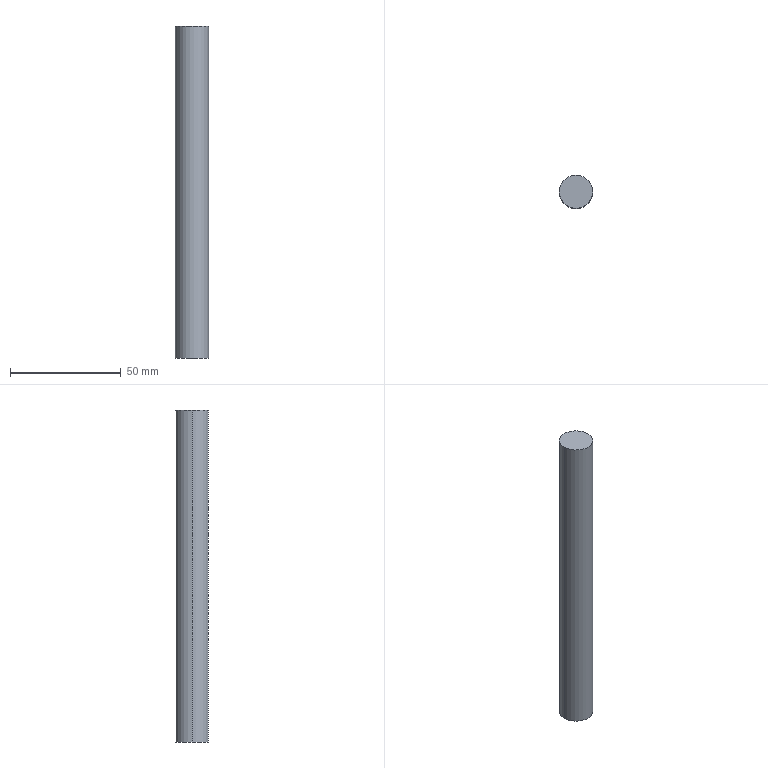Part | SolidWorks | features BaseBody 1 | 1 solid | 4 faces | box 15 x 15 x 150 mm | volume 26507 mm3 | plane 2 | cylinder 2 | commonest cylinder face diameters 15 x2
STEP:
#1=CARTESIAN_POINT('',(-7.5,0.,-75.));
#2=VERTEX_POINT('',#1);
#3=CARTESIAN_POINT('',(7.5,0.,-75.));
#4=VERTEX_POINT('',#3);
#5=CARTESIAN_POINT('',(0.,0.,-75.));
#6=DIRECTION('',(0.,0.,1.));
#7=DIRECTION('',(1.,0.,0.));
#8=AXIS2_PLACEMENT_3D('',#5,#6,#7);
#9=CIRCLE('',#8,7.5);
#10=EDGE_CURVE('',#2,#4,#9,.T.);
#11=ORIENTED_EDGE('',*,*,#10,.F.);
#12=CARTESIAN_POINT('',(0.,0.,-75.));
#13=DIRECTION('',(0.,0.,1.));
#14=DIRECTION('',(1.,0.,0.));
#15=AXIS2_PLACEMENT_3D('',#12,#13,#14);
#16=CIRCLE('',#15,7.5);
#17=EDGE_CURVE('',#4,#2,#16,.T.);
#18=ORIENTED_EDGE('',*,*,#17,.F.);
#19=EDGE_LOOP('',(#11,#18));
#20=FACE_OUTER_BOUND('',#19,.T.);
#21=CARTESIAN_POINT('',(0.,0.,-75.));
#22=DIRECTION('',(0.,0.,1.));
#23=DIRECTION('',(1.,0.,0.));
#24=AXIS2_PLACEMENT_3D('',#21,#22,#23);
#25=PLANE('',#24);
#26=ADVANCED_FACE('',(#20),#25,.F.);
#27=CARTESIAN_POINT('',(-7.5,0.,75.));
#28=VERTEX_POINT('',#27);
#29=CARTESIAN_POINT('',(7.5,0.,75.));
#30=VERTEX_POINT('',#29);
#31=CARTESIAN_POINT('',(0.,0.,75.));
#32=DIRECTION('',(0.,0.,1.));
#33=DIRECTION('',(1.,0.,0.));
#34=AXIS2_PLACEMENT_3D('',#31,#32,#33);
#35=CIRCLE('',#34,7.5);
#36=EDGE_CURVE('',#28,#30,#35,.T.);
#37=ORIENTED_EDGE('',*,*,#36,.T.);
#38=CARTESIAN_POINT('',(0.,0.,75.));
#39=DIRECTION('',(0.,0.,1.));
#40=DIRECTION('',(1.,0.,0.));
#41=AXIS2_PLACEMENT_3D('',#38,#39,#40);
#42=CIRCLE('',#41,7.5);
#43=EDGE_CURVE('',#30,#28,#42,.T.);
#44=ORIENTED_EDGE('',*,*,#43,.T.);
#45=EDGE_LOOP('',(#37,#44));
#46=FACE_OUTER_BOUND('',#45,.T.);
#47=CARTESIAN_POINT('',(0.,0.,75.));
#48=DIRECTION('',(0.,0.,1.));
#49=DIRECTION('',(1.,0.,0.));
#50=AXIS2_PLACEMENT_3D('',#47,#48,#49);
#51=PLANE('',#50);
#52=ADVANCED_FACE('',(#46),#51,.T.);
#53=CARTESIAN_POINT('',(7.5,0.,75.));
#54=DIRECTION('',(0.,0.,-1.));
#55=VECTOR('',#54,1000.);
#56=LINE('',#53,#55);
#57=EDGE_CURVE('',#30,#4,#56,.T.);
#58=ORIENTED_EDGE('',*,*,#57,.F.);
#59=ORIENTED_EDGE('',*,*,#36,.F.);
#60=CARTESIAN_POINT('',(-7.5,0.,75.));
#61=DIRECTION('',(0.,0.,-1.));
#62=VECTOR('',#61,1000.);
#63=LINE('',#60,#62);
#64=EDGE_CURVE('',#28,#2,#63,.T.);
#65=ORIENTED_EDGE('',*,*,#64,.T.);
#66=ORIENTED_EDGE('',*,*,#10,.T.);
#67=EDGE_LOOP('',(#58,#59,#65,#66));
#68=FACE_OUTER_BOUND('',#67,.T.);
#69=CARTESIAN_POINT('',(0.,0.,75.));
#70=DIRECTION('',(0.,0.,-1.));
#71=DIRECTION('',(-1.,0.,0.));
#72=AXIS2_PLACEMENT_3D('',#69,#70,#71);
#73=CYLINDRICAL_SURFACE('',#72,7.5);
#74=ADVANCED_FACE('',(#68),#73,.T.);
#75=ORIENTED_EDGE('',*,*,#43,.F.);
#76=ORIENTED_EDGE('',*,*,#57,.T.);
#77=ORIENTED_EDGE('',*,*,#17,.T.);
#78=ORIENTED_EDGE('',*,*,#64,.F.);
#79=EDGE_LOOP('',(#75,#76,#77,#78));
#80=FACE_OUTER_BOUND('',#79,.T.);
#81=CARTESIAN_POINT('',(0.,0.,75.));
#82=DIRECTION('',(0.,0.,-1.));
#83=DIRECTION('',(-1.,0.,0.));
#84=AXIS2_PLACEMENT_3D('',#81,#82,#83);
#85=CYLINDRICAL_SURFACE('',#84,7.5);
#86=ADVANCED_FACE('',(#80),#85,.T.);
#87=CLOSED_SHELL('',(#26,#52,#74,#86));
#88=MANIFOLD_SOLID_BREP('',#87);
#89=CARTESIAN_POINT('',(0.,0.,0.));
#90=DIRECTION('',(0.,0.,1.));
#91=DIRECTION('',(1.,0.,0.));
#92=AXIS2_PLACEMENT_3D('',#89,#90,#91);
#93=(LENGTH_UNIT()NAMED_UNIT(*)SI_UNIT(.MILLI.,.METRE.));
#94=UNCERTAINTY_MEASURE_WITH_UNIT(LENGTH_MEASURE(0.00001),#93,'','');
#95=(NAMED_UNIT(*)PLANE_ANGLE_UNIT()SI_UNIT($,.RADIAN.));
#96=(NAMED_UNIT(*)SI_UNIT($,.STERADIAN.)SOLID_ANGLE_UNIT());
#97=(GEOMETRIC_REPRESENTATION_CONTEXT(3)GLOBAL_UNCERTAINTY_ASSIGNED_CONTEXT((#94))GLOBAL_UNIT_ASSIGNED_CONTEXT((#93,#95,#96))REPRESENTATION_CONTEXT('',''));
#98=ADVANCED_BREP_SHAPE_REPRESENTATION('',(#88,#92),#97);